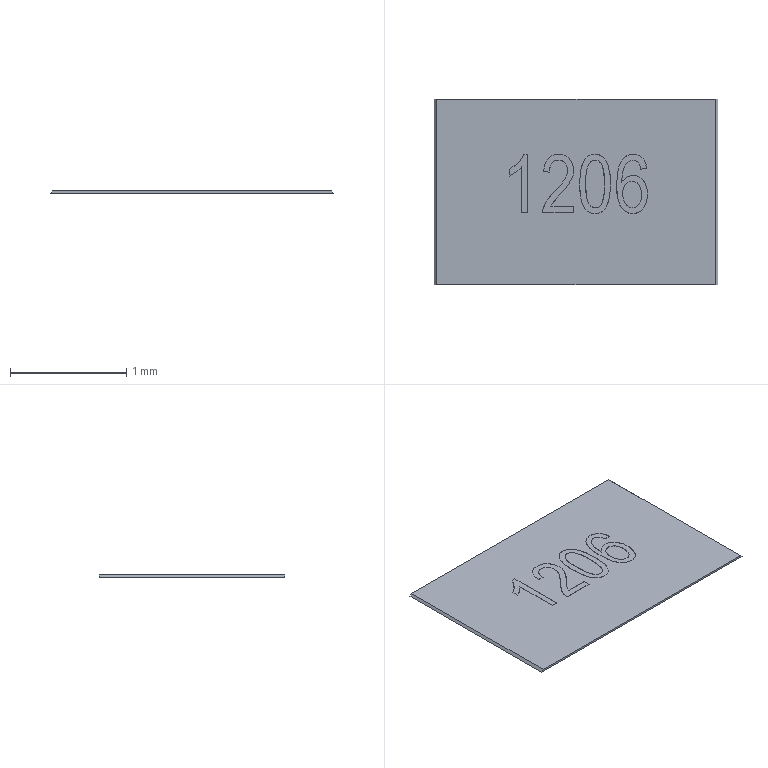Part | STEP file | RJ-USIO-V1_2-220411_23 | 1 solid | 55 faces | box 2.44 x 1.6 x 0.02 mm | volume 0.07724 mm3 | other 33 | plane 22